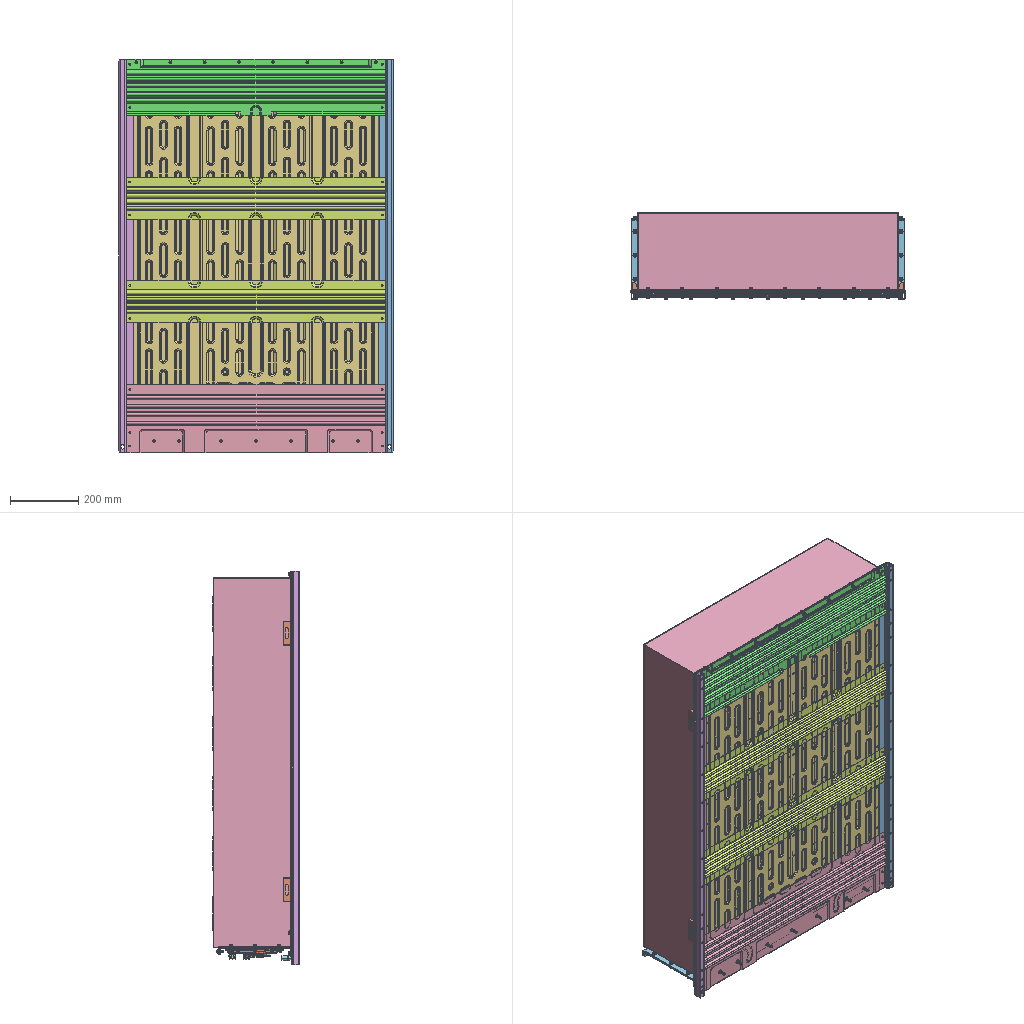Assembly | NX | 111 different items | 547 placed | box 803 x 254 x 1150 mm
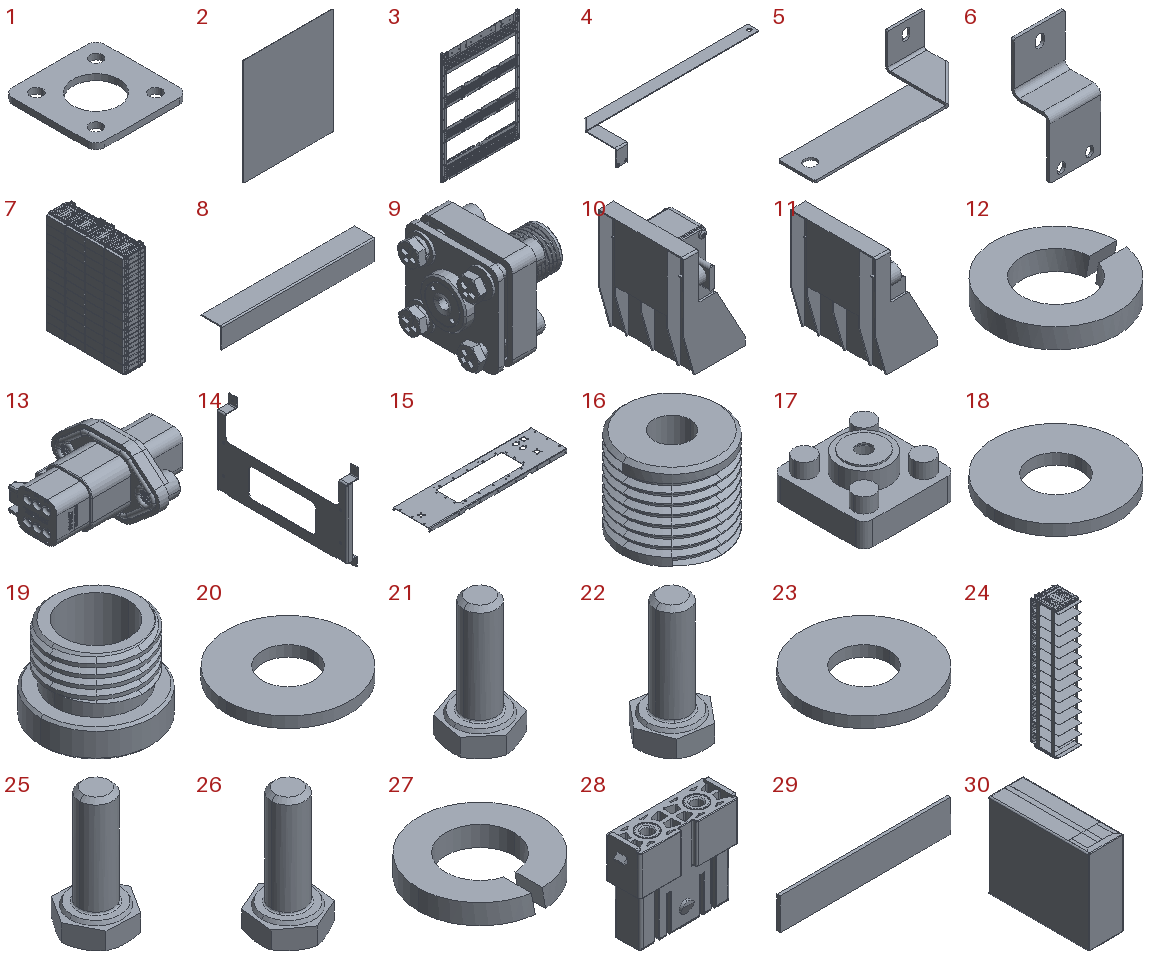Parts list (item | quantity | parent item | size | volume | features):
1 | x1 | in 9 | 31 x 31 x 2 mm | 1418 mm3 | features BREP 1
2 | x48 | in 24, 32 | 173 x 1 x 204 mm | 35284 mm3 | features BREP 1
3 | x1 | in 94 | 800.596 x 20.401 x 1150 mm | 1198428 mm3 | features BREP 5
4 | x1 | in 69 | 457.646 x 111.304 x 46.082 mm | 34595 mm3 | features BREP 1
5 | x1 | in 69 | 138.159 x 50.414 x 31.629 mm | 10937 mm3 | features BREP 1
6 | x1 | in 69 | 36 x 27.2 x 75.856 mm | 6769 mm3 | features BREP 1
7 | x1 | in 96 | - | 139078395 mm3 | features BREP 21
8 | x2 | in 96 | 150 x 20 x 20 mm | 5805 mm3 | features BREP 1
9 | x1 | in 96 | 35.5 x 31 x 31 mm | 13225 mm3 | features BREP 13
10 | x1 | in 96 | 70.8 x 99.662 x 121.2 mm | 149161 mm3 | features BREP 26
11 | x1 | in 10 | 70.8 x 96.5 x 121.2 mm | 76427 mm3 | features BREP 3
12 | x1 | in 9 | 6.78 x 6.78 x 1.1 mm | 26.444 mm3 | features BREP 1
13 | x3 | in 96 | 59.25 x 50 x 31 mm | 25746 mm3 | features BREP 2
14 | x1 | in 55 | 24.9 x 272 x 181.457 mm | 37056 mm3 | features BREP 1
15 | x1 | in 93 | 795 x 208.3 x 21.5 mm | 208004 mm3 | features BREP 1
16 | x1 | in 9 | 13.458 x 13.458 x 11.5 mm | 1248 mm3 | features BREP 1
17 | x1 | in 9 | 31 x 31 x 22.5 mm | 8895 mm3 | features BREP 1
18 | x1 | in 9 | 9 x 9 x 0.8 mm | 41.916 mm3 | features BREP 1
19 | x1 | in 9 | 11.9 x 11.9 x 9 mm | 484.643 mm3 | features BREP 1
20 | x1 | in 9 | 9 x 9 x 0.8 mm | 41.916 mm3 | features BREP 1
21 | x1 | in 9 | 7.602 x 7.957 x 14.8 mm | 249.931 mm3 | features BREP 1
22 | x1 | in 9 | 7.975 x 7.565 x 14.8 mm | 249.934 mm3 | features BREP 1
23 | x1 | in 9 | 9 x 9 x 0.8 mm | 41.916 mm3 | features BREP 1
24 | x2 | in 48 | - | 1550668 mm3 | features BREP 10
25 | x1 | in 9 | 8.074 x 7.182 x 14.8 mm | 249.923 mm3 | features BREP 1
26 | x1 | in 9 | 7.395 x 8.036 x 14.8 mm | 249.924 mm3 | features BREP 1
27 | x1 | in 9 | 6.78 x 6.78 x 1.1 mm | 26.444 mm3 | features BREP 1
28 | x2 | in 48 | 43 x 14 x 36.8 mm | 9836 mm3 | features BREP 2
29 | x32 | in 36, 37, 48, 59 | 160 x 3 x 30 mm | 14400 mm3 | features BREP 1
30 | x52 | in 48, 59 | 71.65 x 206.8 x 174 mm | 2542557 mm3 | features BREP 2
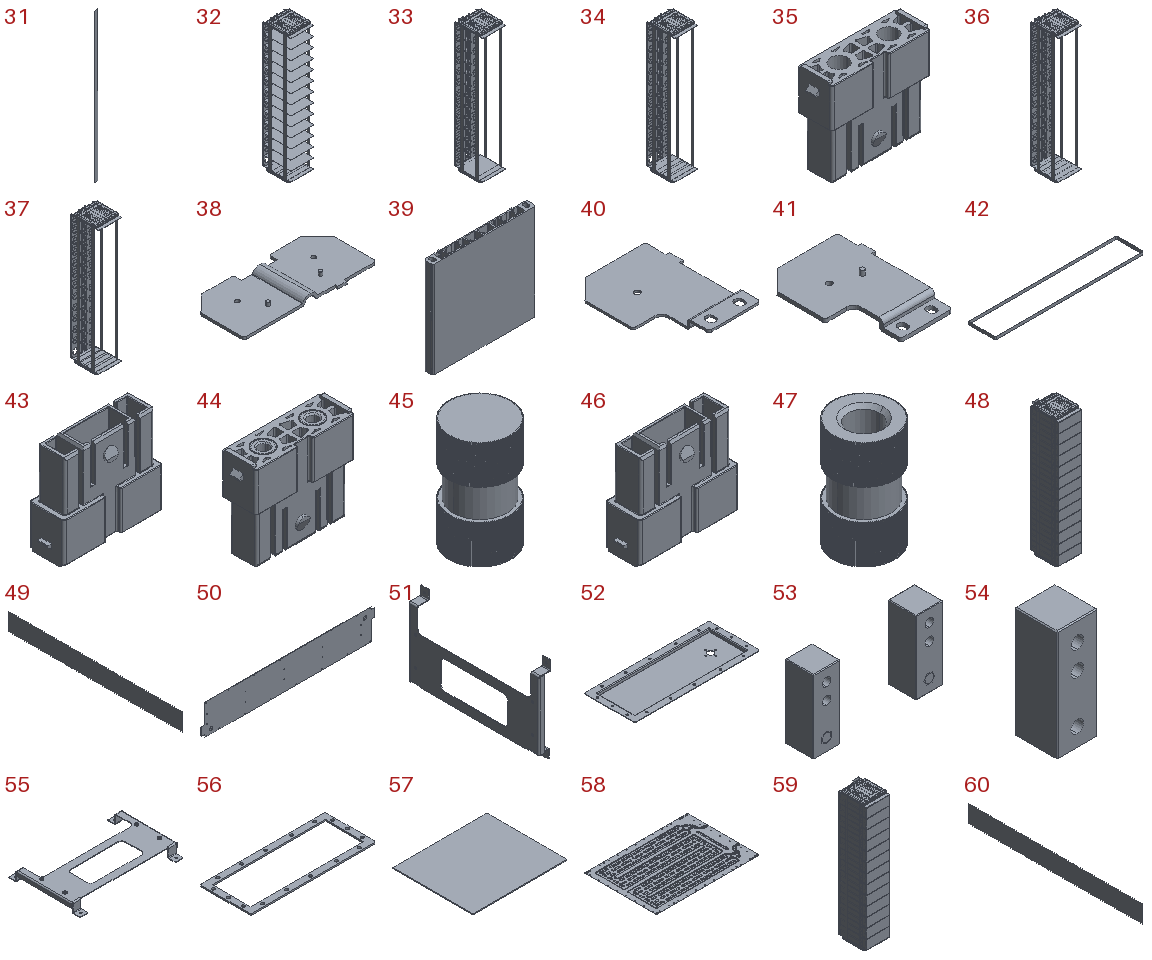31 | x6 | in 48, 59 | 24.5 x 0.5 x 943 mm | 11552 mm3 | features BREP 1
32 | x2 | in 59 | - | 1560221 mm3 | features BREP 9
33 | x2 | in 24 | - | 1127254 mm3 | features BREP 9
34 | x2 | in 32 | - | 1136806 mm3 | features BREP 8
35 | x4 | in 28, 44 | 43 x 14 x 36.8 mm | 8827 mm3 | features BREP 1
36 | x2 | in 33 | - | 1127254 mm3 | features BREP 9
37 | x2 | in 34 | - | 1136806 mm3 | features BREP 8
38 | x48 | in 36, 37 | 125.7 x 58.5 x 8 mm | 16937 mm3 | features BREP 3
39 | x8 | in 36, 37 | 175 x 17.5 x 162.4 mm | 177412 mm3 | features BREP 1
40 | x4 | in 59 | 58.5 x 80.5 x 11 mm | 5793 mm3 | features BREP 1
41 | x4 | in 36 | 58.5 x 80.5 x 11 mm | 9624 mm3 | features BREP 1
42 | x8 | in 36, 37 | 980.9 x 177.8 x 19 mm | 35873 mm3 | features BREP 1
43 | x2 | in 59 | 43 x 14 x 36.8 mm | 9835 mm3 | features BREP 2
44 | x2 | in 48 | 43 x 14 x 36.8 mm | 9836 mm3 | features BREP 2
45 | x8 | in 28, 44 | 8 x 8 x 14 mm | 504.782 mm3 | features BREP 1
46 | x4 | in 43, 90 | 43 x 14 x 36.8 mm | 8827 mm3 | features BREP 1
47 | x8 | in 43, 90 | 8 x 8 x 14 mm | 504.416 mm3 | features BREP 1
48 | x2 | in 7 | - | 34773936 mm3 | features BREP 16
49 | x2 | in 48 | - | - | features BREP 1
50 | x2 | in 48 | 983.7 x 0.7 x 171.2 mm | 81617 mm3 | features BREP 1
51 | x1 | in 14 | 24.9 x 272 x 181.457 mm | 37056 mm3 | features BREP 1
52 | x1 | in 96 | 420 x 170 x 11.5 mm | 119203 mm3 | features BREP 1
53 | x1 | in 111 | 96.925 x 21 x 55.074 mm | 42287 mm3 | features BREP 2
54 | x2 | in 53 | 20 x 21 x 55 mm | 20710 mm3 | features BREP 1
55 | x1 | in 96 | 272 x 181.457 x 26.9 mm | 37450 mm3 | features BREP 2
56 | x1 | in 96 | 420 x 170 x 5 mm | 103610 mm3 | features BREP 1
57 | x8 | in 36, 37 | 204 x 173 x 2 mm | 70582 mm3 | features BREP 1
58 | x1 | in 111 | 1150 x 803 x 4.5 mm | 1042892 mm3 | features BREP 1
59 | x2 | in 7 | - | 34754714 mm3 | features BREP 16
60 | x2 | in 59 | - | - | features BREP 1
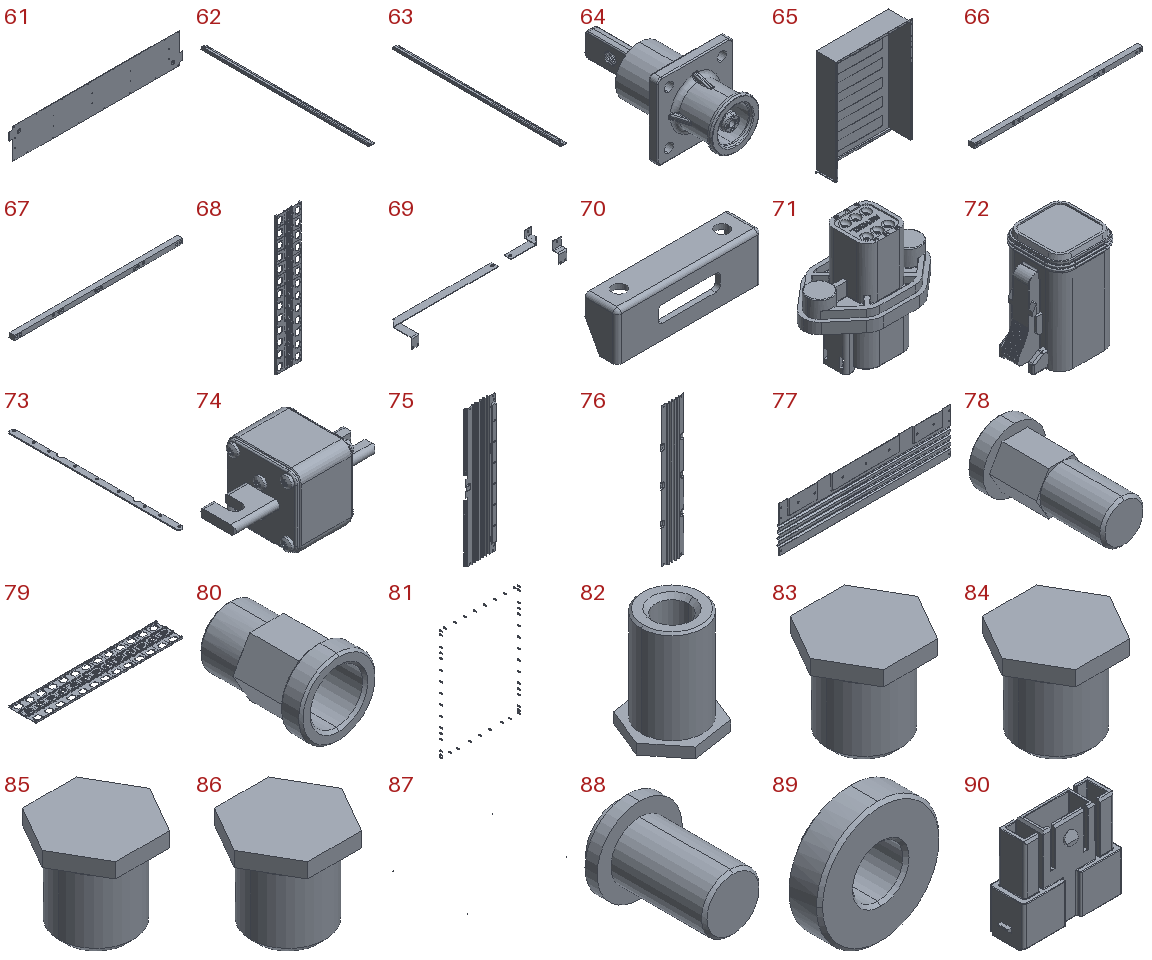61 | x2 | in 59 | 983.7 x 0.7 x 171.2 mm | 81616 mm3 | features BREP 1
62 | x1 | in 3 | 42.999 x 1150 x 20.019 mm | 254430 mm3 | features BREP 1
63 | x1 | in 3 | 43 x 1150 x 20 mm | 254425 mm3 | features BREP 1
64 | x2 | in 96 | 35 x 67.8 x 35 mm | 14088 mm3 | features BREP 1
65 | x1 | in 96 | 798.2 x 228.75 x 1116 mm | 1898468 mm3 | features BREP 1
66 | x2 | in 111 | 731 x 22 x 20 mm | 312679 mm3 | features BREP 2
67 | x2 | in 66 | 731 x 22 x 20 mm | 305206 mm3 | features BREP 1
68 | x4 | in 36, 37 | - | 265096 mm3 | features BREP 1
69 | x1 | in 96 | 676.772 x 128.89 x 75.856 mm | 52301 mm3 | features BREP 3
70 | x4 | in 94 | 70 x 15.5 x 23 mm | 6522 mm3 | features BREP 1
71 | x3 | in 13 | 50 x 31 x 46.3 mm | 15321 mm3 | features BREP 1
72 | x3 | in 13 | 25.459 x 19.5 x 31.65 mm | 10405 mm3 | features BREP 1
73 | x1 | in 94 | 27 x 803 x 5 mm | 101980 mm3 | features BREP 1
74 | x1 | in 10 | 99 x 51 x 51 mm | 72734 mm3 | features BREP 23
75 | x1 | in 3 | 165 x 13.655 x 755.2 mm | 191855 mm3 | features BREP 1
76 | x2 | in 3 | 122 x 13.6 x 755.2 mm | 141700 mm3 | features BREP 1
77 | x1 | in 3 | 755.2 x 13.6 x 200 mm | 214320 mm3 | features BREP 1
78 | x16 | in 93 | 10 x 20 x 10 mm | 454.713 mm3 | features BREP 1
79 | x4 | in 68 | - | 265096 mm3 | features BREP 1
80 | x14 | in 93 | 9 x 13 x 9 mm | 256.908 mm3 | features BREP 1
81 | x1 | in 94 | - | 31916 mm3 | features BREP 1
82 | x12 | in 105 | 7.997 x 7.514 x 10 mm | 235.147 mm3 | features BREP 1
83 | x1 | in 87 | 5.774 x 5 x 5 mm | 67.305 mm3 | features BREP 1
84 | x1 | in 87 | 5.774 x 5 x 5 mm | 67.305 mm3 | features BREP 1
85 | x1 | in 87 | 5.774 x 5 x 5 mm | 67.305 mm3 | features BREP 1
86 | x1 | in 87 | 5.774 x 5 x 5 mm | 67.305 mm3 | features BREP 1
87 | x1 | in 105 | 1047 x 782.008 x 5 mm | 269.222 mm3 | features BREP 4
88 | x8 | in 93 | 7.75 x 10.6 x 7.75 mm | 133.839 mm3 | features BREP 1
89 | x4 | in 55 | 8 x 2.97 x 8 mm | 98.301 mm3 | features BREP 1
90 | x2 | in 59 | 43 x 14 x 36.8 mm | 9835 mm3 | features BREP 2
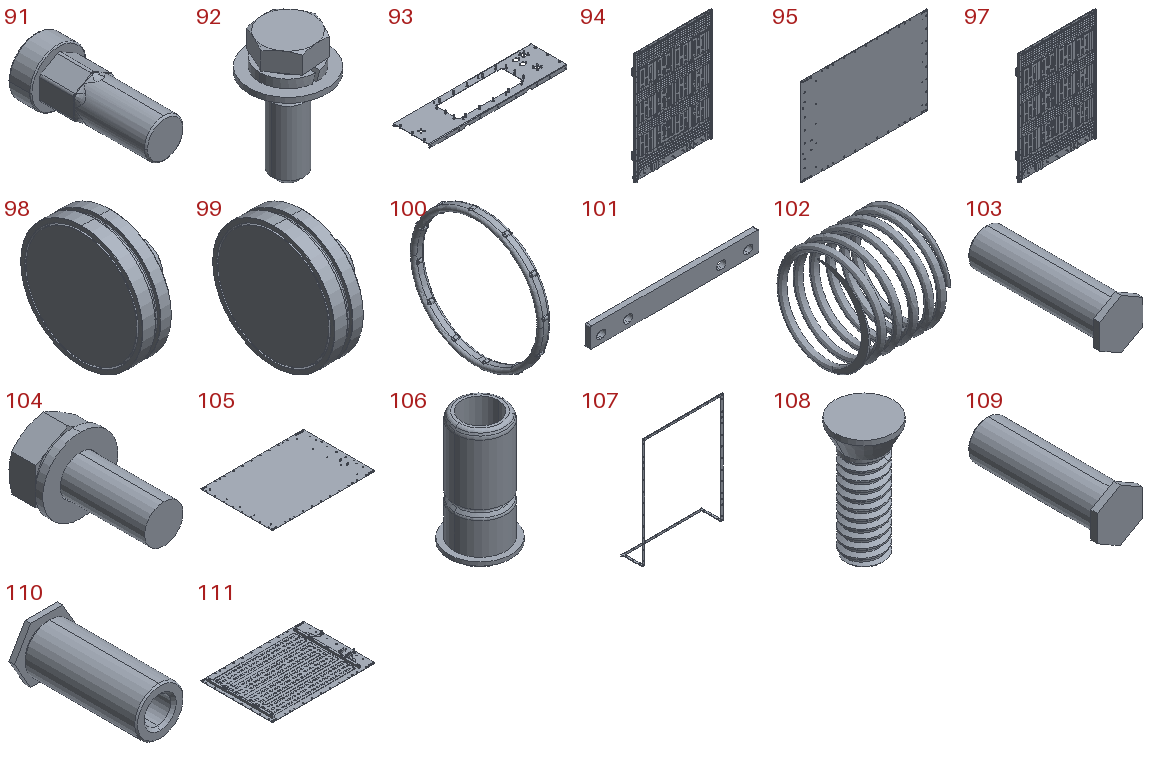91 | x47 | in 81 | 10.002 x 23.005 x 10.001 mm | 588.706 mm3 | features BREP 1
92 | x51 | - | 12 x 12 x 19.5 mm | 603.235 mm3 | features BREP 1
93 | x1 | in 96 | 795 x 210.8 x 37.5 mm | 220520 mm3 | features BREP 5
94 | x1 | in 97 | - | 4182433 mm3 | features BREP 21
95 | x1 | in 105 | 1150 x 1.2 x 803 mm | 1101671 mm3 | features BREP 1
96 | x1 | - | - | - | features BREP 99
97 | x1 | in 96 | - | 4182433 mm3 | features BREP 21
98 | x1 | - | 24.5 x 49.6 x 49.6 mm | 19242 mm3 | features BREP 3
99 | x1 | in 98 | 24.5 x 49.6 x 49.6 mm | 18037 mm3 | features BREP 1
100 | x1 | in 98 | 3.7 x 46.932 x 46.932 mm | 892.47 mm3 | features BREP 1
101 | x3 | in 7 | 125.75 x 4 x 15 mm | 7029 mm3 | features BREP 1
102 | x1 | in 98 | - | 317.43 mm3 | features BREP 1
103 | x2 | in 105 | 7 x 22 x 8.083 mm | 461.807 mm3 | features BREP 1
104 | x4 | - | 7.8 x 13 x 7.8 mm | 254.436 mm3 | features BREP 1
105 | x1 | in 111 | 1150 x 803 x 25.8 mm | 1105685 mm3 | features BREP 7
106 | x2 | in 111 | 17 x 17 x 33 mm | 2358 mm3 | features BREP 1
107 | x1 | in 96 | 798.203 x 215.5 x 1117 mm | 386704 mm3 | features BREP 1
108 | x4 | in 93 | - | 151.707 mm3 | features BREP 1
109 | x2 | in 53 | 7 x 20.5 x 8.083 mm | 432.929 mm3 | features BREP 1
110 | x16 | in 66 | 11.547 x 21.5 x 10 mm | 934.056 mm3 | features BREP 1
111 | x1 | in 94 | - | 2817494 mm3 | features BREP 13